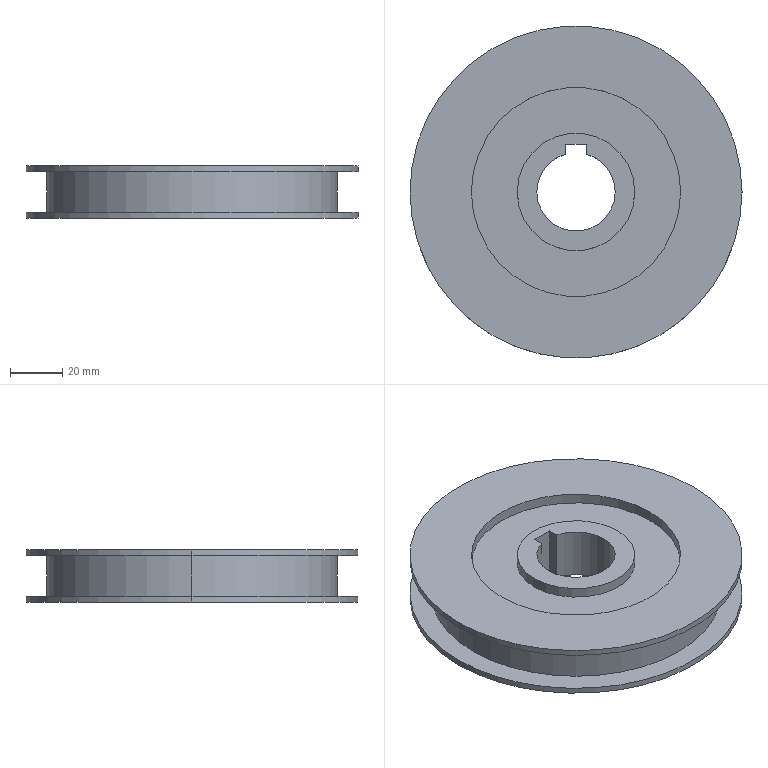Part | STEP file | Pulley 150 belt ha13 v1V11 | 1 solid | 28 faces | box 127 x 127 x 20 mm | volume 165003 mm3 | cylinder 17 | plane 11 | commonest cylinder face diameters 45 x4 80 x4 127 x4 30 x3 111 x2